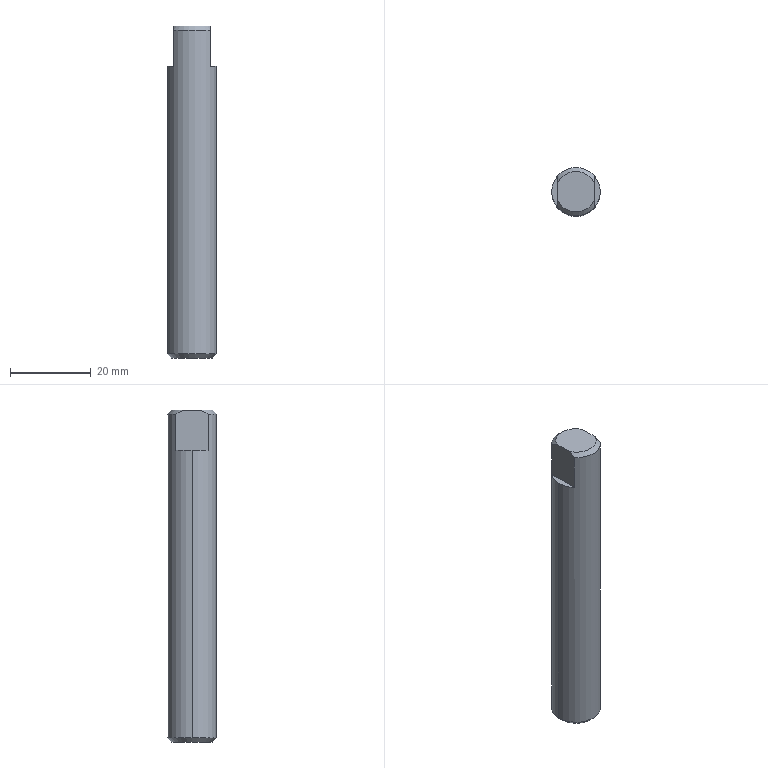Part | STEP file | YCD14007A-08-03.07.07 Sensing Rod | 1 solid | 12 faces | box 12 x 12 x 82 mm | volume 9083 mm3 | plane 6 | cone 4 | cylinder 2 | commonest cylinder face diameters 12 x2
STEP:
#1=CARTESIAN_POINT('',(0.,0.,0.));
#2=DIRECTION('',(0.,0.,1.));
#3=DIRECTION('',(1.,0.,0.));
#4=AXIS2_PLACEMENT_3D('',#1,#2,#3);
#5=CARTESIAN_POINT('',(-5.,0.,0.));
#6=VERTEX_POINT('',#5);
#7=CARTESIAN_POINT('',(5.,0.,0.));
#8=VERTEX_POINT('',#7);
#9=CARTESIAN_POINT('',(0.,0.,0.));
#10=DIRECTION('',(0.,0.,-1.));
#11=DIRECTION('',(1.,0.,0.));
#12=AXIS2_PLACEMENT_3D('',#9,#10,#11);
#13=CIRCLE('',#12,5.);
#14=CARTESIAN_POINT('',(0.,0.,1.));
#15=DIRECTION('',(0.,0.,1.));
#16=DIRECTION('',(1.,0.,0.));
#17=AXIS2_PLACEMENT_3D('',#14,#15,#16);
#18=CONICAL_SURFACE('',#17,6.,0.7854);
#19=CARTESIAN_POINT('',(6.283,-1.));
#20=DIRECTION('',(-1.,0.));
#21=VECTOR('',#20,1.);
#22=LINE('',#19,#21);
#23=(GEOMETRIC_REPRESENTATION_CONTEXT(2)PARAMETRIC_REPRESENTATION_CONTEXT()REPRESENTATION_CONTEXT('',''));
#24=DEFINITIONAL_REPRESENTATION('',(#22),#23);
#25=PCURVE('',#18,#24);
#26=CARTESIAN_POINT('',(0.,0.,0.));
#27=DIRECTION('',(0.,0.,1.));
#28=DIRECTION('',(1.,0.,0.));
#29=AXIS2_PLACEMENT_3D('',#26,#27,#28);
#30=PLANE('',#29);
#31=CARTESIAN_POINT('',(5.,0.));
#32=CARTESIAN_POINT('',(5.,-8.66));
#33=CARTESIAN_POINT('',(-2.5,-4.33));
#34=CARTESIAN_POINT('',(-10.,0.));
#35=CARTESIAN_POINT('',(-2.5,4.33));
#36=CARTESIAN_POINT('',(5.,8.66));
#37=CARTESIAN_POINT('',(5.,0.));
#38=(BOUNDED_CURVE()B_SPLINE_CURVE(2,(#31,#32,#33,#34,#35,#36,#37),.UNSPECIFIED.,.T.,.F.)B_SPLINE_CURVE_WITH_KNOTS((1,2,2,2,2,1),(-2.094,0.,2.094,4.189,6.283,8.378),.UNSPECIFIED.)CURVE()GEOMETRIC_REPRESENTATION_ITEM()RATIONAL_B_SPLINE_CURVE((1.,0.5,1.,0.5,1.,0.5,1.))REPRESENTATION_ITEM(''));
#39=(GEOMETRIC_REPRESENTATION_CONTEXT(2)PARAMETRIC_REPRESENTATION_CONTEXT()REPRESENTATION_CONTEXT('',''));
#40=DEFINITIONAL_REPRESENTATION('',(#38),#39);
#41=PCURVE('',#30,#40);
#42=SURFACE_CURVE('',#13,(#25,#41),.PCURVE_S1.);
#43=EDGE_CURVE('',#6,#8,#42,.T.);
#44=ORIENTED_EDGE('',*,*,#43,.F.);
#45=CARTESIAN_POINT('',(-6.,0.,1.));
#46=VERTEX_POINT('',#45);
#47=CARTESIAN_POINT('',(-6.,0.,1.));
#48=DIRECTION('',(-0.7071,0.,0.7071));
#49=VECTOR('',#48,1.);
#50=LINE('',#47,#49);
#51=CARTESIAN_POINT('',(3.142,0.));
#52=DIRECTION('',(0.,1.));
#53=VECTOR('',#52,1.);
#54=LINE('',#51,#53);
#55=(GEOMETRIC_REPRESENTATION_CONTEXT(2)PARAMETRIC_REPRESENTATION_CONTEXT()REPRESENTATION_CONTEXT('',''));
#56=DEFINITIONAL_REPRESENTATION('',(#54),#55);
#57=PCURVE('',#18,#56);
#58=CARTESIAN_POINT('',(0.,0.,1.));
#59=DIRECTION('',(0.,0.,1.));
#60=DIRECTION('',(1.,0.,0.));
#61=AXIS2_PLACEMENT_3D('',#58,#59,#60);
#62=CONICAL_SURFACE('',#61,6.,0.7854);
#63=CARTESIAN_POINT('',(3.142,0.));
#64=DIRECTION('',(0.,1.));
#65=VECTOR('',#64,1.);
#66=LINE('',#63,#65);
#67=(GEOMETRIC_REPRESENTATION_CONTEXT(2)PARAMETRIC_REPRESENTATION_CONTEXT()REPRESENTATION_CONTEXT('',''));
#68=DEFINITIONAL_REPRESENTATION('',(#66),#67);
#69=PCURVE('',#62,#68);
#70=SURFACE_CURVE('',#50,(#57,#69),.PCURVE_S1.);
#71=EDGE_CURVE('',#6,#46,#70,.T.);
#72=ORIENTED_EDGE('',*,*,#71,.T.);
#73=CARTESIAN_POINT('',(6.,0.,1.));
#74=VERTEX_POINT('',#73);
#75=CARTESIAN_POINT('',(0.,0.,1.));
#76=DIRECTION('',(0.,0.,1.));
#77=DIRECTION('',(1.,0.,0.));
#78=AXIS2_PLACEMENT_3D('',#75,#76,#77);
#79=CIRCLE('',#78,6.);
#80=CARTESIAN_POINT('',(0.,0.));
#81=DIRECTION('',(1.,0.));
#82=VECTOR('',#81,1.);
#83=LINE('',#80,#82);
#84=(GEOMETRIC_REPRESENTATION_CONTEXT(2)PARAMETRIC_REPRESENTATION_CONTEXT()REPRESENTATION_CONTEXT('',''));
#85=DEFINITIONAL_REPRESENTATION('',(#83),#84);
#86=PCURVE('',#18,#85);
#87=CARTESIAN_POINT('',(0.,0.,82.));
#88=DIRECTION('',(0.,0.,-1.));
#89=DIRECTION('',(-1.,0.,0.));
#90=AXIS2_PLACEMENT_3D('',#87,#88,#89);
#91=CYLINDRICAL_SURFACE('',#90,6.);
#92=CARTESIAN_POINT('',(3.142,81.));
#93=DIRECTION('',(-1.,0.));
#94=VECTOR('',#93,1.);
#95=LINE('',#92,#94);
#96=(GEOMETRIC_REPRESENTATION_CONTEXT(2)PARAMETRIC_REPRESENTATION_CONTEXT()REPRESENTATION_CONTEXT('',''));
#97=DEFINITIONAL_REPRESENTATION('',(#95),#96);
#98=PCURVE('',#91,#97);
#99=SURFACE_CURVE('',#79,(#86,#98),.PCURVE_S1.);
#100=EDGE_CURVE('',#74,#46,#99,.T.);
#101=ORIENTED_EDGE('',*,*,#100,.F.);
#102=CARTESIAN_POINT('',(6.,0.,1.));
#103=DIRECTION('',(0.7071,0.,0.7071));
#104=VECTOR('',#103,1.);
#105=LINE('',#102,#104);
#106=CARTESIAN_POINT('',(0.,0.));
#107=DIRECTION('',(0.,1.));
#108=VECTOR('',#107,1.);
#109=LINE('',#106,#108);
#110=(GEOMETRIC_REPRESENTATION_CONTEXT(2)PARAMETRIC_REPRESENTATION_CONTEXT()REPRESENTATION_CONTEXT('',''));
#111=DEFINITIONAL_REPRESENTATION('',(#109),#110);
#112=PCURVE('',#18,#111);
#113=CARTESIAN_POINT('',(6.283,0.));
#114=DIRECTION('',(0.,1.));
#115=VECTOR('',#114,1.);
#116=LINE('',#113,#115);
#117=(GEOMETRIC_REPRESENTATION_CONTEXT(2)PARAMETRIC_REPRESENTATION_CONTEXT()REPRESENTATION_CONTEXT('',''));
#118=DEFINITIONAL_REPRESENTATION('',(#116),#117);
#119=PCURVE('',#62,#118);
#120=SURFACE_CURVE('',#105,(#112,#119),.PCURVE_S1.);
#121=EDGE_CURVE('',#8,#74,#120,.T.);
#122=ORIENTED_EDGE('',*,*,#121,.F.);
#123=EDGE_LOOP('',(#44,#72,#101,#122));
#124=FACE_BOUND('',#123,.T.);
#125=ADVANCED_FACE('',(#124),#18,.T.);
#126=CARTESIAN_POINT('',(4.5,3.969,72.));
#127=VERTEX_POINT('',#126);
#128=CARTESIAN_POINT('',(6.,0.,72.));
#129=VERTEX_POINT('',#128);
#130=CARTESIAN_POINT('',(0.,0.,72.));
#131=DIRECTION('',(0.,0.,-1.));
#132=DIRECTION('',(-1.,0.,0.));
#133=AXIS2_PLACEMENT_3D('',#130,#131,#132);
#134=CIRCLE('',#133,6.);
#135=CARTESIAN_POINT('',(0.,10.));
#136=DIRECTION('',(1.,0.));
#137=VECTOR('',#136,1.);
#138=LINE('',#135,#137);
#139=(GEOMETRIC_REPRESENTATION_CONTEXT(2)PARAMETRIC_REPRESENTATION_CONTEXT()REPRESENTATION_CONTEXT('',''));
#140=DEFINITIONAL_REPRESENTATION('',(#138),#139);
#141=PCURVE('',#91,#140);
#142=CARTESIAN_POINT('',(6.,-32.,72.));
#143=DIRECTION('',(0.,0.,-1.));
#144=DIRECTION('',(-1.,0.,0.));
#145=AXIS2_PLACEMENT_3D('',#142,#143,#144);
#146=PLANE('',#145);
#147=CARTESIAN_POINT('',(6.,32.));
#148=DIRECTION('',(1.,0.));
#149=AXIS2_PLACEMENT_2D('',#147,#148);
#150=CIRCLE('',#149,6.);
#151=(GEOMETRIC_REPRESENTATION_CONTEXT(2)PARAMETRIC_REPRESENTATION_CONTEXT()REPRESENTATION_CONTEXT('',''));
#152=DEFINITIONAL_REPRESENTATION('',(#150),#151);
#153=PCURVE('',#146,#152);
#154=SURFACE_CURVE('',#134,(#141,#153),.PCURVE_S1.);
#155=EDGE_CURVE('',#127,#129,#154,.T.);
#156=ORIENTED_EDGE('',*,*,#155,.T.);
#157=CARTESIAN_POINT('',(6.,0.,82.));
#158=DIRECTION('',(0.,0.,-1.));
#159=VECTOR('',#158,1.);
#160=LINE('',#157,#159);
#161=CARTESIAN_POINT('',(3.142,0.));
#162=DIRECTION('',(0.,1.));
#163=VECTOR('',#162,1.);
#164=LINE('',#161,#163);
#165=(GEOMETRIC_REPRESENTATION_CONTEXT(2)PARAMETRIC_REPRESENTATION_CONTEXT()REPRESENTATION_CONTEXT('',''));
#166=DEFINITIONAL_REPRESENTATION('',(#164),#165);
#167=PCURVE('',#91,#166);
#168=CARTESIAN_POINT('',(0.,0.,82.));
#169=DIRECTION('',(0.,0.,-1.));
#170=DIRECTION('',(-1.,0.,0.));
#171=AXIS2_PLACEMENT_3D('',#168,#169,#170);
#172=CYLINDRICAL_SURFACE('',#171,6.);
#173=CARTESIAN_POINT('',(3.142,0.));
#174=DIRECTION('',(0.,1.));
#175=VECTOR('',#174,1.);
#176=LINE('',#173,#175);
#177=(GEOMETRIC_REPRESENTATION_CONTEXT(2)PARAMETRIC_REPRESENTATION_CONTEXT()REPRESENTATION_CONTEXT('',''));
#178=DEFINITIONAL_REPRESENTATION('',(#176),#177);
#179=PCURVE('',#172,#178);
#180=SURFACE_CURVE('',#160,(#167,#179),.PCURVE_S1.);
#181=EDGE_CURVE('',#129,#74,#180,.T.);
#182=ORIENTED_EDGE('',*,*,#181,.T.);
#183=ORIENTED_EDGE('',*,*,#100,.T.);
#184=CARTESIAN_POINT('',(-6.,0.,72.));
#185=VERTEX_POINT('',#184);
#186=CARTESIAN_POINT('',(-6.,0.,82.));
#187=DIRECTION('',(0.,0.,-1.));
#188=VECTOR('',#187,1.);
#189=LINE('',#186,#188);
#190=CARTESIAN_POINT('',(0.,0.));
#191=DIRECTION('',(0.,1.));
#192=VECTOR('',#191,1.);
#193=LINE('',#190,#192);
#194=(GEOMETRIC_REPRESENTATION_CONTEXT(2)PARAMETRIC_REPRESENTATION_CONTEXT()REPRESENTATION_CONTEXT('',''));
#195=DEFINITIONAL_REPRESENTATION('',(#193),#194);
#196=PCURVE('',#91,#195);
#197=CARTESIAN_POINT('',(6.283,0.));
#198=DIRECTION('',(0.,1.));
#199=VECTOR('',#198,1.);
#200=LINE('',#197,#199);
#201=(GEOMETRIC_REPRESENTATION_CONTEXT(2)PARAMETRIC_REPRESENTATION_CONTEXT()REPRESENTATION_CONTEXT('',''));
#202=DEFINITIONAL_REPRESENTATION('',(#200),#201);
#203=PCURVE('',#172,#202);
#204=SURFACE_CURVE('',#189,(#196,#203),.PCURVE_S1.);
#205=EDGE_CURVE('',#185,#46,#204,.T.);
#206=ORIENTED_EDGE('',*,*,#205,.F.);
#207=CARTESIAN_POINT('',(-4.5,3.969,72.));
#208=VERTEX_POINT('',#207);
#209=CARTESIAN_POINT('',(0.,0.,72.));
#210=DIRECTION('',(0.,0.,-1.));
#211=DIRECTION('',(-1.,0.,0.));
#212=AXIS2_PLACEMENT_3D('',#209,#210,#211);
#213=CIRCLE('',#212,6.);
#214=CARTESIAN_POINT('',(0.,10.));
#215=DIRECTION('',(1.,0.));
#216=VECTOR('',#215,1.);
#217=LINE('',#214,#216);
#218=(GEOMETRIC_REPRESENTATION_CONTEXT(2)PARAMETRIC_REPRESENTATION_CONTEXT()REPRESENTATION_CONTEXT('',''));
#219=DEFINITIONAL_REPRESENTATION('',(#217),#218);
#220=PCURVE('',#91,#219);
#221=CARTESIAN_POINT('',(-6.,-32.,72.));
#222=DIRECTION('',(0.,0.,-1.));
#223=DIRECTION('',(-1.,0.,0.));
#224=AXIS2_PLACEMENT_3D('',#221,#222,#223);
#225=PLANE('',#224);
#226=CARTESIAN_POINT('',(-6.,32.));
#227=DIRECTION('',(1.,0.));
#228=AXIS2_PLACEMENT_2D('',#226,#227);
#229=CIRCLE('',#228,6.);
#230=(GEOMETRIC_REPRESENTATION_CONTEXT(2)PARAMETRIC_REPRESENTATION_CONTEXT()REPRESENTATION_CONTEXT('',''));
#231=DEFINITIONAL_REPRESENTATION('',(#229),#230);
#232=PCURVE('',#225,#231);
#233=SURFACE_CURVE('',#213,(#220,#232),.PCURVE_S1.);
#234=EDGE_CURVE('',#185,#208,#233,.T.);
#235=ORIENTED_EDGE('',*,*,#234,.T.);
#236=CARTESIAN_POINT('',(-4.5,3.969,81.));
#237=VERTEX_POINT('',#236);
#238=CARTESIAN_POINT('',(-4.5,3.969,82.));
#239=DIRECTION('',(0.,0.,1.));
#240=VECTOR('',#239,1.);
#241=LINE('',#238,#240);
#242=CARTESIAN_POINT('',(0.7227,0.));
#243=DIRECTION('',(0.,-1.));
#244=VECTOR('',#243,1.);
#245=LINE('',#242,#244);
#246=(GEOMETRIC_REPRESENTATION_CONTEXT(2)PARAMETRIC_REPRESENTATION_CONTEXT()REPRESENTATION_CONTEXT('',''));
#247=DEFINITIONAL_REPRESENTATION('',(#245),#246);
#248=PCURVE('',#91,#247);
#249=CARTESIAN_POINT('',(-4.5,-32.,82.));
#250=DIRECTION('',(1.,0.,0.));
#251=DIRECTION('',(0.,0.,-1.));
#252=AXIS2_PLACEMENT_3D('',#249,#250,#251);
#253=PLANE('',#252);
#254=CARTESIAN_POINT('',(0.,35.969));
#255=DIRECTION('',(-1.,0.));
#256=VECTOR('',#255,1.);
#257=LINE('',#254,#256);
#258=(GEOMETRIC_REPRESENTATION_CONTEXT(2)PARAMETRIC_REPRESENTATION_CONTEXT()REPRESENTATION_CONTEXT('',''));
#259=DEFINITIONAL_REPRESENTATION('',(#257),#258);
#260=PCURVE('',#253,#259);
#261=SURFACE_CURVE('',#241,(#248,#260),.PCURVE_S1.);
#262=EDGE_CURVE('',#208,#237,#261,.T.);
#263=ORIENTED_EDGE('',*,*,#262,.T.);
#264=CARTESIAN_POINT('',(4.5,3.969,81.));
#265=VERTEX_POINT('',#264);
#266=CARTESIAN_POINT('',(0.,0.,81.));
#267=DIRECTION('',(0.,0.,-1.));
#268=DIRECTION('',(1.,0.,0.));
#269=AXIS2_PLACEMENT_3D('',#266,#267,#268);
#270=CIRCLE('',#269,6.);
#271=CARTESIAN_POINT('',(-3.142,1.));
#272=DIRECTION('',(1.,0.));
#273=VECTOR('',#272,1.);
#274=LINE('',#271,#273);
#275=(GEOMETRIC_REPRESENTATION_CONTEXT(2)PARAMETRIC_REPRESENTATION_CONTEXT()REPRESENTATION_CONTEXT('',''));
#276=DEFINITIONAL_REPRESENTATION('',(#274),#275);
#277=PCURVE('',#91,#276);
#278=CARTESIAN_POINT('',(0.,0.,82.));
#279=DIRECTION('',(0.,0.,-1.));
#280=DIRECTION('',(-1.,0.,0.));
#281=AXIS2_PLACEMENT_3D('',#278,#279,#280);
#282=CONICAL_SURFACE('',#281,5.,0.7854);
#283=CARTESIAN_POINT('',(-3.142,1.));
#284=DIRECTION('',(1.,0.));
#285=VECTOR('',#284,1.);
#286=LINE('',#283,#285);
#287=(GEOMETRIC_REPRESENTATION_CONTEXT(2)PARAMETRIC_REPRESENTATION_CONTEXT()REPRESENTATION_CONTEXT('',''));
#288=DEFINITIONAL_REPRESENTATION('',(#286),#287);
#289=PCURVE('',#282,#288);
#290=SURFACE_CURVE('',#270,(#277,#289),.PCURVE_S1.);
#291=EDGE_CURVE('',#237,#265,#290,.T.);
#292=ORIENTED_EDGE('',*,*,#291,.T.);
#293=CARTESIAN_POINT('',(4.5,3.969,82.));
#294=DIRECTION('',(0.,0.,-1.));
#295=VECTOR('',#294,1.);
#296=LINE('',#293,#295);
#297=CARTESIAN_POINT('',(2.419,0.));
#298=DIRECTION('',(0.,1.));
#299=VECTOR('',#298,1.);
#300=LINE('',#297,#299);
#301=(GEOMETRIC_REPRESENTATION_CONTEXT(2)PARAMETRIC_REPRESENTATION_CONTEXT()REPRESENTATION_CONTEXT('',''));
#302=DEFINITIONAL_REPRESENTATION('',(#300),#301);
#303=PCURVE('',#91,#302);
#304=CARTESIAN_POINT('',(4.5,-32.,82.));
#305=DIRECTION('',(-1.,0.,0.));
#306=DIRECTION('',(0.,0.,1.));
#307=AXIS2_PLACEMENT_3D('',#304,#305,#306);
#308=PLANE('',#307);
#309=CARTESIAN_POINT('',(0.,35.969));
#310=DIRECTION('',(-1.,0.));
#311=VECTOR('',#310,1.);
#312=LINE('',#309,#311);
#313=(GEOMETRIC_REPRESENTATION_CONTEXT(2)PARAMETRIC_REPRESENTATION_CONTEXT()REPRESENTATION_CONTEXT('',''));
#314=DEFINITIONAL_REPRESENTATION('',(#312),#313);
#315=PCURVE('',#308,#314);
#316=SURFACE_CURVE('',#296,(#303,#315),.PCURVE_S1.);
#317=EDGE_CURVE('',#265,#127,#316,.T.);
#318=ORIENTED_EDGE('',*,*,#317,.T.);
#319=EDGE_LOOP('',(#156,#182,#183,#206,#235,#263,#292,#318));
#320=FACE_BOUND('',#319,.T.);
#321=ADVANCED_FACE('',(#320),#91,.T.);
#322=CARTESIAN_POINT('',(-4.5,-3.969,81.));
#323=VERTEX_POINT('',#322);
#324=CARTESIAN_POINT('',(-4.5,-2.179,82.));
#325=VERTEX_POINT('',#324);
#326=CARTESIAN_POINT('',(-4.5,-3.969,81.));
#327=CARTESIAN_POINT('',(-4.5,-3.685,81.187));
#328=CARTESIAN_POINT('',(-4.5,-3.396,81.367));
#329=CARTESIAN_POINT('',(-4.5,-2.802,81.704));
#330=CARTESIAN_POINT('',(-4.5,-2.497,81.862));
#331=CARTESIAN_POINT('',(-4.5,-2.179,82.));
#332=B_SPLINE_CURVE_WITH_KNOTS('',3,(#326,#327,#328,#329,#330,#331),.UNSPECIFIED.,.F.,.F.,(4,2,4),(0.01115,0.01218,0.0132),.UNSPECIFIED.);
#333=CARTESIAN_POINT('',(0.,0.,82.));
#334=DIRECTION('',(0.,0.,-1.));
#335=DIRECTION('',(-1.,0.,0.));
#336=AXIS2_PLACEMENT_3D('',#333,#334,#335);
#337=CONICAL_SURFACE('',#336,5.,0.7854);
#338=CARTESIAN_POINT('',(5.56,1.));
#339=CARTESIAN_POINT('',(5.564,0.983));
#340=CARTESIAN_POINT('',(5.57,0.949));
#341=CARTESIAN_POINT('',(5.58,0.8984));
#342=CARTESIAN_POINT('',(5.59,0.8483));
#343=CARTESIAN_POINT('',(5.601,0.7986));
#344=CARTESIAN_POINT('',(5.611,0.7493));
#345=CARTESIAN_POINT('',(5.622,0.7005));
#346=CARTESIAN_POINT('',(5.633,0.6522));
#347=CARTESIAN_POINT('',(5.645,0.6044));
#348=CARTESIAN_POINT('',(5.656,0.557));
#349=CARTESIAN_POINT('',(5.668,0.5103));
#350=CARTESIAN_POINT('',(5.68,0.464));
#351=CARTESIAN_POINT('',(5.692,0.4184));
#352=CARTESIAN_POINT('',(5.705,0.3733));
#353=CARTESIAN_POINT('',(5.718,0.3288));
#354=CARTESIAN_POINT('',(5.731,0.285));
#355=CARTESIAN_POINT('',(5.745,0.2419));
#356=CARTESIAN_POINT('',(5.758,0.1996));
#357=CARTESIAN_POINT('',(5.772,0.1579));
#358=CARTESIAN_POINT('',(5.787,0.1171));
#359=CARTESIAN_POINT('',(5.802,0.07713));
#360=CARTESIAN_POINT('',(5.817,0.03803));
#361=CARTESIAN_POINT('',(5.827,0.01257));
#362=CARTESIAN_POINT('',(5.832,0.));
#363=B_SPLINE_CURVE_WITH_KNOTS('',3,(#338,#339,#340,#341,#342,#343,#344,#345,#346,#347,#348,#349,#350,#351,#352,#353,#354,#355,#356,#357,#358,#359,#360,#361,#362),.UNSPECIFIED.,.F.,.F.,(4,1,1,1,1,1,1,1,1,1,1,1,1,1,1,1,1,1,1,1,1,1,4),(0.01115,0.01125,0.01134,0.01143,0.01152,0.01162,0.01171,0.0118,0.0119,0.01199,0.01208,0.01218,0.01227,0.01236,0.01245,0.01255,0.01264,0.01273,0.01283,0.01292,0.01301,0.01311,0.0132),.QUASI_UNIFORM_KNOTS.);
#364=(GEOMETRIC_REPRESENTATION_CONTEXT(2)PARAMETRIC_REPRESENTATION_CONTEXT()REPRESENTATION_CONTEXT('',''));
#365=DEFINITIONAL_REPRESENTATION('',(#363),#364);
#366=PCURVE('',#337,#365);
#367=CARTESIAN_POINT('',(1.,28.031));
#368=CARTESIAN_POINT('',(0.8125,28.315));
#369=CARTESIAN_POINT('',(0.6326,28.604));
#370=CARTESIAN_POINT('',(0.2957,29.198));
#371=CARTESIAN_POINT('',(0.1383,29.503));
#372=CARTESIAN_POINT('',(0.,29.821));
#373=B_SPLINE_CURVE_WITH_KNOTS('',3,(#367,#368,#369,#370,#371,#372),.UNSPECIFIED.,.F.,.F.,(4,2,4),(0.01115,0.01218,0.0132),.UNSPECIFIED.);
#374=(GEOMETRIC_REPRESENTATION_CONTEXT(2)PARAMETRIC_REPRESENTATION_CONTEXT()REPRESENTATION_CONTEXT('',''));
#375=DEFINITIONAL_REPRESENTATION('',(#373),#374);
#376=PCURVE('',#253,#375);
#377=SURFACE_CURVE('',#332,(#366,#376),.PCURVE_S1.);
#378=EDGE_CURVE('',#323,#325,#377,.T.);
#379=ORIENTED_EDGE('',*,*,#378,.F.);
#380=CARTESIAN_POINT('',(4.5,-3.969,81.));
#381=VERTEX_POINT('',#380);
#382=CARTESIAN_POINT('',(0.,0.,81.));
#383=DIRECTION('',(0.,0.,-1.));
#384=DIRECTION('',(1.,0.,0.));
#385=AXIS2_PLACEMENT_3D('',#382,#383,#384);
#386=CIRCLE('',#385,6.);
#387=CARTESIAN_POINT('',(3.142,1.));
#388=DIRECTION('',(1.,0.));
#389=VECTOR('',#388,1.);
#390=LINE('',#387,#389);
#391=(GEOMETRIC_REPRESENTATION_CONTEXT(2)PARAMETRIC_REPRESENTATION_CONTEXT()REPRESENTATION_CONTEXT('',''));
#392=DEFINITIONAL_REPRESENTATION('',(#390),#391);
#393=PCURVE('',#337,#392);
#394=CARTESIAN_POINT('',(3.142,1.));
#395=DIRECTION('',(1.,0.));
#396=VECTOR('',#395,1.);
#397=LINE('',#394,#396);
#398=(GEOMETRIC_REPRESENTATION_CONTEXT(2)PARAMETRIC_REPRESENTATION_CONTEXT()REPRESENTATION_CONTEXT('',''));
#399=DEFINITIONAL_REPRESENTATION('',(#397),#398);
#400=PCURVE('',#172,#399);
#401=SURFACE_CURVE('',#386,(#393,#400),.PCURVE_S1.);
#402=EDGE_CURVE('',#381,#323,#401,.T.);
#403=ORIENTED_EDGE('',*,*,#402,.F.);
#404=CARTESIAN_POINT('',(4.5,-2.179,82.));
#405=VERTEX_POINT('',#404);
#406=CARTESIAN_POINT('',(4.5,-2.179,82.));
#407=CARTESIAN_POINT('',(4.5,-2.492,81.864));
#408=CARTESIAN_POINT('',(4.5,-2.796,81.708));
#409=CARTESIAN_POINT('',(4.5,-3.391,81.371));
#410=CARTESIAN_POINT('',(4.5,-3.683,81.189));
#411=CARTESIAN_POINT('',(4.5,-3.969,81.));
#412=B_SPLINE_CURVE_WITH_KNOTS('',3,(#406,#407,#408,#409,#410,#411),.UNSPECIFIED.,.F.,.F.,(4,2,4),(0.01766,0.01868,0.0197),.UNSPECIFIED.);
#413=CARTESIAN_POINT('',(3.593,0.));
#414=CARTESIAN_POINT('',(3.598,0.01239));
#415=CARTESIAN_POINT('',(3.608,0.03749));
#416=CARTESIAN_POINT('',(3.623,0.07609));
#417=CARTESIAN_POINT('',(3.637,0.1156));
#418=CARTESIAN_POINT('',(3.652,0.156));
#419=CARTESIAN_POINT('',(3.666,0.1972));
#420=CARTESIAN_POINT('',(3.679,0.2392));
#421=CARTESIAN_POINT('',(3.693,0.2821));
#422=CARTESIAN_POINT('',(3.706,0.3256));
#423=CARTESIAN_POINT('',(3.719,0.3699));
#424=CARTESIAN_POINT('',(3.731,0.4149));
#425=CARTESIAN_POINT('',(3.744,0.4606));
#426=CARTESIAN_POINT('',(3.756,0.5069));
#427=CARTESIAN_POINT('',(3.768,0.5539));
#428=CARTESIAN_POINT('',(3.78,0.6014));
#429=CARTESIAN_POINT('',(3.791,0.6496));
#430=CARTESIAN_POINT('',(3.802,0.6982));
#431=CARTESIAN_POINT('',(3.813,0.7474));
#432=CARTESIAN_POINT('',(3.824,0.7971));
#433=CARTESIAN_POINT('',(3.834,0.8472));
#434=CARTESIAN_POINT('',(3.844,0.8977));
#435=CARTESIAN_POINT('',(3.855,0.9487));
#436=CARTESIAN_POINT('',(3.861,0.9828));
#437=CARTESIAN_POINT('',(3.864,1.));
#438=B_SPLINE_CURVE_WITH_KNOTS('',3,(#413,#414,#415,#416,#417,#418,#419,#420,#421,#422,#423,#424,#425,#426,#427,#428,#429,#430,#431,#432,#433,#434,#435,#436,#437),.UNSPECIFIED.,.F.,.F.,(4,1,1,1,1,1,1,1,1,1,1,1,1,1,1,1,1,1,1,1,1,1,4),(0.01766,0.01776,0.01785,0.01794,0.01804,0.01813,0.01822,0.01831,0.01841,0.0185,0.01859,0.01868,0.01878,0.01887,0.01896,0.01905,0.01915,0.01924,0.01933,0.01942,0.01952,0.01961,0.0197),.QUASI_UNIFORM_KNOTS.);
#439=(GEOMETRIC_REPRESENTATION_CONTEXT(2)PARAMETRIC_REPRESENTATION_CONTEXT()REPRESENTATION_CONTEXT('',''));
#440=DEFINITIONAL_REPRESENTATION('',(#438),#439);
#441=PCURVE('',#337,#440);
#442=CARTESIAN_POINT('',(0.,29.821));
#443=CARTESIAN_POINT('',(-0.1363,29.508));
#444=CARTESIAN_POINT('',(-0.2921,29.204));
#445=CARTESIAN_POINT('',(-0.6294,28.609));
#446=CARTESIAN_POINT('',(-0.8113,28.317));
#447=CARTESIAN_POINT('',(-1.,28.031));
#448=B_SPLINE_CURVE_WITH_KNOTS('',3,(#442,#443,#444,#445,#446,#447),.UNSPECIFIED.,.F.,.F.,(4,2,4),(0.01766,0.01868,0.0197),.UNSPECIFIED.);
#449=(GEOMETRIC_REPRESENTATION_CONTEXT(2)PARAMETRIC_REPRESENTATION_CONTEXT()REPRESENTATION_CONTEXT('',''));
#450=DEFINITIONAL_REPRESENTATION('',(#448),#449);
#451=PCURVE('',#308,#450);
#452=SURFACE_CURVE('',#412,(#441,#451),.PCURVE_S1.);
#453=EDGE_CURVE('',#405,#381,#452,.T.);
#454=ORIENTED_EDGE('',*,*,#453,.F.);
#455=CARTESIAN_POINT('',(0.,0.,82.));
#456=DIRECTION('',(0.,0.,1.));
#457=DIRECTION('',(1.,0.,0.));
#458=AXIS2_PLACEMENT_3D('',#455,#456,#457);
#459=CIRCLE('',#458,5.);
#460=CARTESIAN_POINT('',(9.425,0.));
#461=DIRECTION('',(-1.,0.));
#462=VECTOR('',#461,1.);
#463=LINE('',#460,#462);
#464=(GEOMETRIC_REPRESENTATION_CONTEXT(2)PARAMETRIC_REPRESENTATION_CONTEXT()REPRESENTATION_CONTEXT('',''));
#465=DEFINITIONAL_REPRESENTATION('',(#463),#464);
#466=PCURVE('',#337,#465);
#467=CARTESIAN_POINT('',(0.,0.,82.));
#468=DIRECTION('',(0.,0.,1.));
#469=DIRECTION('',(1.,0.,0.));
#470=AXIS2_PLACEMENT_3D('',#467,#468,#469);
#471=PLANE('',#470);
#472=CARTESIAN_POINT('',(0.,0.));
#473=DIRECTION('',(1.,0.));
#474=AXIS2_PLACEMENT_2D('',#472,#473);
#475=CIRCLE('',#474,5.);
#476=(GEOMETRIC_REPRESENTATION_CONTEXT(2)PARAMETRIC_REPRESENTATION_CONTEXT()REPRESENTATION_CONTEXT('',''));
#477=DEFINITIONAL_REPRESENTATION('',(#475),#476);
#478=PCURVE('',#471,#477);
#479=SURFACE_CURVE('',#459,(#466,#478),.PCURVE_S1.);
#480=EDGE_CURVE('',#325,#405,#479,.T.);
#481=ORIENTED_EDGE('',*,*,#480,.F.);
#482=EDGE_LOOP('',(#379,#403,#454,#481));
#483=FACE_BOUND('',#482,.T.);
#484=ADVANCED_FACE('',(#483),#337,.T.);
#485=ORIENTED_EDGE('',*,*,#181,.F.);
#486=CARTESIAN_POINT('',(4.5,-3.969,72.));
#487=VERTEX_POINT('',#486);
#488=CARTESIAN_POINT('',(0.,0.,72.));
#489=DIRECTION('',(0.,0.,-1.));
#490=DIRECTION('',(-1.,0.,0.));
#491=AXIS2_PLACEMENT_3D('',#488,#489,#490);
#492=CIRCLE('',#491,6.);
#493=CARTESIAN_POINT('',(0.,10.));
#494=DIRECTION('',(1.,0.));
#495=VECTOR('',#494,1.);
#496=LINE('',#493,#495);
#497=(GEOMETRIC_REPRESENTATION_CONTEXT(2)PARAMETRIC_REPRESENTATION_CONTEXT()REPRESENTATION_CONTEXT('',''));
#498=DEFINITIONAL_REPRESENTATION('',(#496),#497);
#499=PCURVE('',#172,#498);
#500=CARTESIAN_POINT('',(6.,32.));
#501=DIRECTION('',(1.,0.));
#502=AXIS2_PLACEMENT_2D('',#500,#501);
#503=CIRCLE('',#502,6.);
#504=(GEOMETRIC_REPRESENTATION_CONTEXT(2)PARAMETRIC_REPRESENTATION_CONTEXT()REPRESENTATION_CONTEXT('',''));
#505=DEFINITIONAL_REPRESENTATION('',(#503),#504);
#506=PCURVE('',#146,#505);
#507=SURFACE_CURVE('',#492,(#499,#506),.PCURVE_S1.);
#508=EDGE_CURVE('',#129,#487,#507,.T.);
#509=ORIENTED_EDGE('',*,*,#508,.T.);
#510=CARTESIAN_POINT('',(4.5,-3.969,82.));
#511=DIRECTION('',(0.,0.,1.));
#512=VECTOR('',#511,1.);
#513=LINE('',#510,#512);
#514=CARTESIAN_POINT('',(3.864,0.));
#515=DIRECTION('',(0.,-1.));
#516=VECTOR('',#515,1.);
#517=LINE('',#514,#516);
#518=(GEOMETRIC_REPRESENTATION_CONTEXT(2)PARAMETRIC_REPRESENTATION_CONTEXT()REPRESENTATION_CONTEXT('',''));
#519=DEFINITIONAL_REPRESENTATION('',(#517),#518);
#520=PCURVE('',#172,#519);
#521=CARTESIAN_POINT('',(0.,28.031));
#522=DIRECTION('',(1.,0.));
#523=VECTOR('',#522,1.);
#524=LINE('',#521,#523);
#525=(GEOMETRIC_REPRESENTATION_CONTEXT(2)PARAMETRIC_REPRESENTATION_CONTEXT()REPRESENTATION_CONTEXT('',''));
#526=DEFINITIONAL_REPRESENTATION('',(#524),#525);
#527=PCURVE('',#308,#526);
#528=SURFACE_CURVE('',#513,(#520,#527),.PCURVE_S1.);
#529=EDGE_CURVE('',#487,#381,#528,.T.);
#530=ORIENTED_EDGE('',*,*,#529,.T.);
#531=ORIENTED_EDGE('',*,*,#402,.T.);
#532=CARTESIAN_POINT('',(-4.5,-3.969,72.));
#533=VERTEX_POINT('',#532);
#534=CARTESIAN_POINT('',(-4.5,-3.969,82.));
#535=DIRECTION('',(0.,0.,-1.));
#536=VECTOR('',#535,1.);
#537=LINE('',#534,#536);
#538=CARTESIAN_POINT('',(5.56,0.));
#539=DIRECTION('',(0.,1.));
#540=VECTOR('',#539,1.);
#541=LINE('',#538,#540);
#542=(GEOMETRIC_REPRESENTATION_CONTEXT(2)PARAMETRIC_REPRESENTATION_CONTEXT()REPRESENTATION_CONTEXT('',''));
#543=DEFINITIONAL_REPRESENTATION('',(#541),#542);
#544=PCURVE('',#172,#543);
#545=CARTESIAN_POINT('',(0.,28.031));
#546=DIRECTION('',(1.,0.));
#547=VECTOR('',#546,1.);
#548=LINE('',#545,#547);
#549=(GEOMETRIC_REPRESENTATION_CONTEXT(2)PARAMETRIC_REPRESENTATION_CONTEXT()REPRESENTATION_CONTEXT('',''));
#550=DEFINITIONAL_REPRESENTATION('',(#548),#549);
#551=PCURVE('',#253,#550);
#552=SURFACE_CURVE('',#537,(#544,#551),.PCURVE_S1.);
#553=EDGE_CURVE('',#323,#533,#552,.T.);
#554=ORIENTED_EDGE('',*,*,#553,.T.);
#555=CARTESIAN_POINT('',(0.,0.,72.));
#556=DIRECTION('',(0.,0.,-1.));
#557=DIRECTION('',(-1.,0.,0.));
#558=AXIS2_PLACEMENT_3D('',#555,#556,#557);
#559=CIRCLE('',#558,6.);
#560=CARTESIAN_POINT('',(0.,10.));
#561=DIRECTION('',(1.,0.));
#562=VECTOR('',#561,1.);
#563=LINE('',#560,#562);
#564=(GEOMETRIC_REPRESENTATION_CONTEXT(2)PARAMETRIC_REPRESENTATION_CONTEXT()REPRESENTATION_CONTEXT('',''));
#565=DEFINITIONAL_REPRESENTATION('',(#563),#564);
#566=PCURVE('',#172,#565);
#567=CARTESIAN_POINT('',(-6.,32.));
#568=DIRECTION('',(1.,0.));
#569=AXIS2_PLACEMENT_2D('',#567,#568);
#570=CIRCLE('',#569,6.);
#571=(GEOMETRIC_REPRESENTATION_CONTEXT(2)PARAMETRIC_REPRESENTATION_CONTEXT()REPRESENTATION_CONTEXT('',''));
#572=DEFINITIONAL_REPRESENTATION('',(#570),#571);
#573=PCURVE('',#225,#572);
#574=SURFACE_CURVE('',#559,(#566,#573),.PCURVE_S1.);
#575=EDGE_CURVE('',#533,#185,#574,.T.);
#576=ORIENTED_EDGE('',*,*,#575,.T.);
#577=ORIENTED_EDGE('',*,*,#205,.T.);
#578=CARTESIAN_POINT('',(0.,0.,1.));
#579=DIRECTION('',(0.,0.,1.));
#580=DIRECTION('',(1.,0.,0.));
#581=AXIS2_PLACEMENT_3D('',#578,#579,#580);
#582=CIRCLE('',#581,6.);
#583=CARTESIAN_POINT('',(9.425,81.));
#584=DIRECTION('',(-1.,0.));
#585=VECTOR('',#584,1.);
#586=LINE('',#583,#585);
#587=(GEOMETRIC_REPRESENTATION_CONTEXT(2)PARAMETRIC_REPRESENTATION_CONTEXT()REPRESENTATION_CONTEXT('',''));
#588=DEFINITIONAL_REPRESENTATION('',(#586),#587);
#589=PCURVE('',#172,#588);
#590=CARTESIAN_POINT('',(0.,0.));
#591=DIRECTION('',(1.,0.));
#592=VECTOR('',#591,1.);
#593=LINE('',#590,#592);
#594=(GEOMETRIC_REPRESENTATION_CONTEXT(2)PARAMETRIC_REPRESENTATION_CONTEXT()REPRESENTATION_CONTEXT('',''));
#595=DEFINITIONAL_REPRESENTATION('',(#593),#594);
#596=PCURVE('',#62,#595);
#597=SURFACE_CURVE('',#582,(#589,#596),.PCURVE_S1.);
#598=EDGE_CURVE('',#46,#74,#597,.T.);
#599=ORIENTED_EDGE('',*,*,#598,.T.);
#600=EDGE_LOOP('',(#485,#509,#530,#531,#554,#576,#577,#599));
#601=FACE_BOUND('',#600,.T.);
#602=ADVANCED_FACE('',(#601),#172,.T.);
#603=CARTESIAN_POINT('',(-4.5,2.179,82.));
#604=VERTEX_POINT('',#603);
#605=CARTESIAN_POINT('',(-4.5,-32.,82.));
#606=DIRECTION('',(0.,1.,0.));
#607=VECTOR('',#606,1.);
#608=LINE('',#605,#607);
#609=CARTESIAN_POINT('',(-4.5,-32.));
#610=DIRECTION('',(0.,1.));
#611=VECTOR('',#610,1.);
#612=LINE('',#609,#611);
#613=(GEOMETRIC_REPRESENTATION_CONTEXT(2)PARAMETRIC_REPRESENTATION_CONTEXT()REPRESENTATION_CONTEXT('',''));
#614=DEFINITIONAL_REPRESENTATION('',(#612),#613);
#615=PCURVE('',#471,#614);
#616=CARTESIAN_POINT('',(0.,0.));
#617=DIRECTION('',(0.,1.));
#618=VECTOR('',#617,1.);
#619=LINE('',#616,#618);
#620=(GEOMETRIC_REPRESENTATION_CONTEXT(2)PARAMETRIC_REPRESENTATION_CONTEXT()REPRESENTATION_CONTEXT('',''));
#621=DEFINITIONAL_REPRESENTATION('',(#619),#620);
#622=PCURVE('',#253,#621);
#623=SURFACE_CURVE('',#608,(#615,#622),.PCURVE_S1.);
#624=EDGE_CURVE('',#325,#604,#623,.T.);
#625=ORIENTED_EDGE('',*,*,#624,.F.);
#626=ORIENTED_EDGE('',*,*,#480,.T.);
#627=CARTESIAN_POINT('',(4.5,2.179,82.));
#628=VERTEX_POINT('',#627);
#629=CARTESIAN_POINT('',(4.5,-32.,82.));
#630=DIRECTION('',(0.,1.,0.));
#631=VECTOR('',#630,1.);
#632=LINE('',#629,#631);
#633=CARTESIAN_POINT('',(4.5,-32.));
#634=DIRECTION('',(0.,1.));
#635=VECTOR('',#634,1.);
#636=LINE('',#633,#635);
#637=(GEOMETRIC_REPRESENTATION_CONTEXT(2)PARAMETRIC_REPRESENTATION_CONTEXT()REPRESENTATION_CONTEXT('',''));
#638=DEFINITIONAL_REPRESENTATION('',(#636),#637);
#639=PCURVE('',#471,#638);
#640=CARTESIAN_POINT('',(0.,0.));
#641=DIRECTION('',(0.,1.));
#642=VECTOR('',#641,1.);
#643=LINE('',#640,#642);
#644=(GEOMETRIC_REPRESENTATION_CONTEXT(2)PARAMETRIC_REPRESENTATION_CONTEXT()REPRESENTATION_CONTEXT('',''));
#645=DEFINITIONAL_REPRESENTATION('',(#643),#644);
#646=PCURVE('',#308,#645);
#647=SURFACE_CURVE('',#632,(#639,#646),.PCURVE_S1.);
#648=EDGE_CURVE('',#405,#628,#647,.T.);
#649=ORIENTED_EDGE('',*,*,#648,.T.);
#650=CARTESIAN_POINT('',(0.,0.,82.));
#651=DIRECTION('',(0.,0.,1.));
#652=DIRECTION('',(1.,0.,0.));
#653=AXIS2_PLACEMENT_3D('',#650,#651,#652);
#654=CIRCLE('',#653,5.);
#655=CARTESIAN_POINT('',(0.,0.));
#656=DIRECTION('',(1.,0.));
#657=AXIS2_PLACEMENT_2D('',#655,#656);
#658=CIRCLE('',#657,5.);
#659=(GEOMETRIC_REPRESENTATION_CONTEXT(2)PARAMETRIC_REPRESENTATION_CONTEXT()REPRESENTATION_CONTEXT('',''));
#660=DEFINITIONAL_REPRESENTATION('',(#658),#659);
#661=PCURVE('',#471,#660);
#662=CARTESIAN_POINT('',(3.142,0.));
#663=DIRECTION('',(-1.,0.));
#664=VECTOR('',#663,1.);
#665=LINE('',#662,#664);
#666=(GEOMETRIC_REPRESENTATION_CONTEXT(2)PARAMETRIC_REPRESENTATION_CONTEXT()REPRESENTATION_CONTEXT('',''));
#667=DEFINITIONAL_REPRESENTATION('',(#665),#666);
#668=PCURVE('',#282,#667);
#669=SURFACE_CURVE('',#654,(#661,#668),.PCURVE_S1.);
#670=EDGE_CURVE('',#628,#604,#669,.T.);
#671=ORIENTED_EDGE('',*,*,#670,.T.);
#672=EDGE_LOOP('',(#625,#626,#649,#671));
#673=FACE_BOUND('',#672,.T.);
#674=ADVANCED_FACE('',(#673),#471,.T.);
#675=CARTESIAN_POINT('',(0.,0.,0.));
#676=DIRECTION('',(0.,0.,-1.));
#677=DIRECTION('',(1.,0.,0.));
#678=AXIS2_PLACEMENT_3D('',#675,#676,#677);
#679=CIRCLE('',#678,5.);
#680=CARTESIAN_POINT('',(5.,0.));
#681=CARTESIAN_POINT('',(5.,-8.66));
#682=CARTESIAN_POINT('',(-2.5,-4.33));
#683=CARTESIAN_POINT('',(-10.,0.));
#684=CARTESIAN_POINT('',(-2.5,4.33));
#685=CARTESIAN_POINT('',(5.,8.66));
#686=CARTESIAN_POINT('',(5.,0.));
#687=(BOUNDED_CURVE()B_SPLINE_CURVE(2,(#680,#681,#682,#683,#684,#685,#686),.UNSPECIFIED.,.T.,.F.)B_SPLINE_CURVE_WITH_KNOTS((1,2,2,2,2,1),(-2.094,0.,2.094,4.189,6.283,8.378),.UNSPECIFIED.)CURVE()GEOMETRIC_REPRESENTATION_ITEM()RATIONAL_B_SPLINE_CURVE((1.,0.5,1.,0.5,1.,0.5,1.))REPRESENTATION_ITEM(''));
#688=(GEOMETRIC_REPRESENTATION_CONTEXT(2)PARAMETRIC_REPRESENTATION_CONTEXT()REPRESENTATION_CONTEXT('',''));
#689=DEFINITIONAL_REPRESENTATION('',(#687),#688);
#690=PCURVE('',#30,#689);
#691=CARTESIAN_POINT('',(6.283,-1.));
#692=DIRECTION('',(-1.,0.));
#693=VECTOR('',#692,1.);
#694=LINE('',#691,#693);
#695=(GEOMETRIC_REPRESENTATION_CONTEXT(2)PARAMETRIC_REPRESENTATION_CONTEXT()REPRESENTATION_CONTEXT('',''));
#696=DEFINITIONAL_REPRESENTATION('',(#694),#695);
#697=PCURVE('',#62,#696);
#698=SURFACE_CURVE('',#679,(#690,#697),.PCURVE_S1.);
#699=EDGE_CURVE('',#8,#6,#698,.T.);
#700=ORIENTED_EDGE('',*,*,#699,.T.);
#701=ORIENTED_EDGE('',*,*,#43,.T.);
#702=EDGE_LOOP('',(#700,#701));
#703=FACE_BOUND('',#702,.T.);
#704=ADVANCED_FACE('',(#703),#30,.F.);
#705=ORIENTED_EDGE('',*,*,#71,.F.);
#706=ORIENTED_EDGE('',*,*,#699,.F.);
#707=ORIENTED_EDGE('',*,*,#121,.T.);
#708=ORIENTED_EDGE('',*,*,#598,.F.);
#709=EDGE_LOOP('',(#705,#706,#707,#708));
#710=FACE_BOUND('',#709,.T.);
#711=ADVANCED_FACE('',(#710),#62,.T.);
#712=CARTESIAN_POINT('',(-4.5,2.179,82.));
#713=CARTESIAN_POINT('',(-4.5,2.492,81.864));
#714=CARTESIAN_POINT('',(-4.5,2.796,81.708));
#715=CARTESIAN_POINT('',(-4.5,3.391,81.371));
#716=CARTESIAN_POINT('',(-4.5,3.683,81.189));
#717=CARTESIAN_POINT('',(-4.5,3.969,81.));
#718=B_SPLINE_CURVE_WITH_KNOTS('',3,(#712,#713,#714,#715,#716,#717),.UNSPECIFIED.,.F.,.F.,(4,2,4),(0.01766,0.01868,0.0197),.UNSPECIFIED.);
#719=CARTESIAN_POINT('',(0.451,0.));
#720=CARTESIAN_POINT('',(0.4561,0.01239));
#721=CARTESIAN_POINT('',(0.4663,0.03749));
#722=CARTESIAN_POINT('',(0.4812,0.07609));
#723=CARTESIAN_POINT('',(0.4958,0.1156));
#724=CARTESIAN_POINT('',(0.51,0.156));
#725=CARTESIAN_POINT('',(0.524,0.1972));
#726=CARTESIAN_POINT('',(0.5378,0.2392));
#727=CARTESIAN_POINT('',(0.5512,0.2821));
#728=CARTESIAN_POINT('',(0.5644,0.3256));
#729=CARTESIAN_POINT('',(0.5773,0.3699));
#730=CARTESIAN_POINT('',(0.5899,0.4149));
#731=CARTESIAN_POINT('',(0.6023,0.4606));
#732=CARTESIAN_POINT('',(0.6144,0.5069));
#733=CARTESIAN_POINT('',(0.6263,0.5539));
#734=CARTESIAN_POINT('',(0.6379,0.6014));
#735=CARTESIAN_POINT('',(0.6493,0.6496));
#736=CARTESIAN_POINT('',(0.6605,0.6982));
#737=CARTESIAN_POINT('',(0.6714,0.7474));
#738=CARTESIAN_POINT('',(0.6822,0.7971));
#739=CARTESIAN_POINT('',(0.6926,0.8472));
#740=CARTESIAN_POINT('',(0.7029,0.8977));
#741=CARTESIAN_POINT('',(0.7129,0.9487));
#742=CARTESIAN_POINT('',(0.7195,0.9828));
#743=CARTESIAN_POINT('',(0.7227,1.));
#744=B_SPLINE_CURVE_WITH_KNOTS('',3,(#719,#720,#721,#722,#723,#724,#725,#726,#727,#728,#729,#730,#731,#732,#733,#734,#735,#736,#737,#738,#739,#740,#741,#742,#743),.UNSPECIFIED.,.F.,.F.,(4,1,1,1,1,1,1,1,1,1,1,1,1,1,1,1,1,1,1,1,1,1,4),(0.01766,0.01776,0.01785,0.01794,0.01804,0.01813,0.01822,0.01831,0.01841,0.0185,0.01859,0.01868,0.01878,0.01887,0.01896,0.01905,0.01915,0.01924,0.01933,0.01942,0.01952,0.01961,0.0197),.QUASI_UNIFORM_KNOTS.);
#745=(GEOMETRIC_REPRESENTATION_CONTEXT(2)PARAMETRIC_REPRESENTATION_CONTEXT()REPRESENTATION_CONTEXT('',''));
#746=DEFINITIONAL_REPRESENTATION('',(#744),#745);
#747=PCURVE('',#282,#746);
#748=CARTESIAN_POINT('',(0.,34.179));
#749=CARTESIAN_POINT('',(0.1363,34.492));
#750=CARTESIAN_POINT('',(0.2921,34.796));
#751=CARTESIAN_POINT('',(0.6294,35.391));
#752=CARTESIAN_POINT('',(0.8113,35.683));
#753=CARTESIAN_POINT('',(1.,35.969));
#754=B_SPLINE_CURVE_WITH_KNOTS('',3,(#748,#749,#750,#751,#752,#753),.UNSPECIFIED.,.F.,.F.,(4,2,4),(0.01766,0.01868,0.0197),.UNSPECIFIED.);
#755=(GEOMETRIC_REPRESENTATION_CONTEXT(2)PARAMETRIC_REPRESENTATION_CONTEXT()REPRESENTATION_CONTEXT('',''));
#756=DEFINITIONAL_REPRESENTATION('',(#754),#755);
#757=PCURVE('',#253,#756);
#758=SURFACE_CURVE('',#718,(#747,#757),.PCURVE_S1.);
#759=EDGE_CURVE('',#604,#237,#758,.T.);
#760=ORIENTED_EDGE('',*,*,#759,.F.);
#761=ORIENTED_EDGE('',*,*,#670,.F.);
#762=CARTESIAN_POINT('',(4.5,3.969,81.));
#763=CARTESIAN_POINT('',(4.5,3.685,81.187));
#764=CARTESIAN_POINT('',(4.5,3.396,81.367));
#765=CARTESIAN_POINT('',(4.5,2.802,81.704));
#766=CARTESIAN_POINT('',(4.5,2.497,81.862));
#767=CARTESIAN_POINT('',(4.5,2.179,82.));
#768=B_SPLINE_CURVE_WITH_KNOTS('',3,(#762,#763,#764,#765,#766,#767),.UNSPECIFIED.,.F.,.F.,(4,2,4),(0.01115,0.01218,0.0132),.UNSPECIFIED.);
#769=CARTESIAN_POINT('',(2.419,1.));
#770=CARTESIAN_POINT('',(2.422,0.983));
#771=CARTESIAN_POINT('',(2.429,0.949));
#772=CARTESIAN_POINT('',(2.439,0.8984));
#773=CARTESIAN_POINT('',(2.449,0.8483));
#774=CARTESIAN_POINT('',(2.459,0.7986));
#775=CARTESIAN_POINT('',(2.47,0.7493));
#776=CARTESIAN_POINT('',(2.481,0.7005));
#777=CARTESIAN_POINT('',(2.492,0.6522));
#778=CARTESIAN_POINT('',(2.503,0.6044));
#779=CARTESIAN_POINT('',(2.515,0.557));
#780=CARTESIAN_POINT('',(2.526,0.5103));
#781=CARTESIAN_POINT('',(2.538,0.464));
#782=CARTESIAN_POINT('',(2.551,0.4184));
#783=CARTESIAN_POINT('',(2.563,0.3733));
#784=CARTESIAN_POINT('',(2.576,0.3288));
#785=CARTESIAN_POINT('',(2.589,0.285));
#786=CARTESIAN_POINT('',(2.603,0.2419));
#787=CARTESIAN_POINT('',(2.617,0.1996));
#788=CARTESIAN_POINT('',(2.631,0.1579));
#789=CARTESIAN_POINT('',(2.645,0.1171));
#790=CARTESIAN_POINT('',(2.66,0.07713));
#791=CARTESIAN_POINT('',(2.675,0.03803));
#792=CARTESIAN_POINT('',(2.685,0.01257));
#793=CARTESIAN_POINT('',(2.691,0.));
#794=B_SPLINE_CURVE_WITH_KNOTS('',3,(#769,#770,#771,#772,#773,#774,#775,#776,#777,#778,#779,#780,#781,#782,#783,#784,#785,#786,#787,#788,#789,#790,#791,#792,#793),.UNSPECIFIED.,.F.,.F.,(4,1,1,1,1,1,1,1,1,1,1,1,1,1,1,1,1,1,1,1,1,1,4),(0.01115,0.01125,0.01134,0.01143,0.01152,0.01162,0.01171,0.0118,0.0119,0.01199,0.01208,0.01218,0.01227,0.01236,0.01245,0.01255,0.01264,0.01273,0.01283,0.01292,0.01301,0.01311,0.0132),.QUASI_UNIFORM_KNOTS.);
#795=(GEOMETRIC_REPRESENTATION_CONTEXT(2)PARAMETRIC_REPRESENTATION_CONTEXT()REPRESENTATION_CONTEXT('',''));
#796=DEFINITIONAL_REPRESENTATION('',(#794),#795);
#797=PCURVE('',#282,#796);
#798=CARTESIAN_POINT('',(-1.,35.969));
#799=CARTESIAN_POINT('',(-0.8125,35.685));
#800=CARTESIAN_POINT('',(-0.6326,35.396));
#801=CARTESIAN_POINT('',(-0.2957,34.802));
#802=CARTESIAN_POINT('',(-0.1383,34.497));
#803=CARTESIAN_POINT('',(0.,34.179));
#804=B_SPLINE_CURVE_WITH_KNOTS('',3,(#798,#799,#800,#801,#802,#803),.UNSPECIFIED.,.F.,.F.,(4,2,4),(0.01115,0.01218,0.0132),.UNSPECIFIED.);
#805=(GEOMETRIC_REPRESENTATION_CONTEXT(2)PARAMETRIC_REPRESENTATION_CONTEXT()REPRESENTATION_CONTEXT('',''));
#806=DEFINITIONAL_REPRESENTATION('',(#804),#805);
#807=PCURVE('',#308,#806);
#808=SURFACE_CURVE('',#768,(#797,#807),.PCURVE_S1.);
#809=EDGE_CURVE('',#265,#628,#808,.T.);
#810=ORIENTED_EDGE('',*,*,#809,.F.);
#811=ORIENTED_EDGE('',*,*,#291,.F.);
#812=EDGE_LOOP('',(#760,#761,#810,#811));
#813=FACE_BOUND('',#812,.T.);
#814=ADVANCED_FACE('',(#813),#282,.T.);
#815=CARTESIAN_POINT('',(4.5,-32.,72.));
#816=DIRECTION('',(0.,1.,0.));
#817=VECTOR('',#816,1.);
#818=LINE('',#815,#817);
#819=CARTESIAN_POINT('',(1.5,0.));
#820=DIRECTION('',(0.,1.));
#821=VECTOR('',#820,1.);
#822=LINE('',#819,#821);
#823=(GEOMETRIC_REPRESENTATION_CONTEXT(2)PARAMETRIC_REPRESENTATION_CONTEXT()REPRESENTATION_CONTEXT('',''));
#824=DEFINITIONAL_REPRESENTATION('',(#822),#823);
#825=PCURVE('',#146,#824);
#826=CARTESIAN_POINT('',(-10.,0.));
#827=DIRECTION('',(0.,1.));
#828=VECTOR('',#827,1.);
#829=LINE('',#826,#828);
#830=(GEOMETRIC_REPRESENTATION_CONTEXT(2)PARAMETRIC_REPRESENTATION_CONTEXT()REPRESENTATION_CONTEXT('',''));
#831=DEFINITIONAL_REPRESENTATION('',(#829),#830);
#832=PCURVE('',#308,#831);
#833=SURFACE_CURVE('',#818,(#825,#832),.PCURVE_S1.);
#834=EDGE_CURVE('',#487,#127,#833,.T.);
#835=ORIENTED_EDGE('',*,*,#834,.F.);
#836=ORIENTED_EDGE('',*,*,#508,.F.);
#837=ORIENTED_EDGE('',*,*,#155,.F.);
#838=EDGE_LOOP('',(#835,#836,#837));
#839=FACE_BOUND('',#838,.T.);
#840=ADVANCED_FACE('',(#839),#146,.F.);
#841=ORIENTED_EDGE('',*,*,#809,.T.);
#842=ORIENTED_EDGE('',*,*,#648,.F.);
#843=ORIENTED_EDGE('',*,*,#453,.T.);
#844=ORIENTED_EDGE('',*,*,#529,.F.);
#845=ORIENTED_EDGE('',*,*,#834,.T.);
#846=ORIENTED_EDGE('',*,*,#317,.F.);
#847=EDGE_LOOP('',(#841,#842,#843,#844,#845,#846));
#848=FACE_BOUND('',#847,.T.);
#849=ADVANCED_FACE('',(#848),#308,.F.);
#850=ORIENTED_EDGE('',*,*,#575,.F.);
#851=CARTESIAN_POINT('',(-4.5,-32.,72.));
#852=DIRECTION('',(0.,1.,0.));
#853=VECTOR('',#852,1.);
#854=LINE('',#851,#853);
#855=CARTESIAN_POINT('',(-1.5,0.));
#856=DIRECTION('',(0.,1.));
#857=VECTOR('',#856,1.);
#858=LINE('',#855,#857);
#859=(GEOMETRIC_REPRESENTATION_CONTEXT(2)PARAMETRIC_REPRESENTATION_CONTEXT()REPRESENTATION_CONTEXT('',''));
#860=DEFINITIONAL_REPRESENTATION('',(#858),#859);
#861=PCURVE('',#225,#860);
#862=CARTESIAN_POINT('',(10.,0.));
#863=DIRECTION('',(0.,1.));
#864=VECTOR('',#863,1.);
#865=LINE('',#862,#864);
#866=(GEOMETRIC_REPRESENTATION_CONTEXT(2)PARAMETRIC_REPRESENTATION_CONTEXT()REPRESENTATION_CONTEXT('',''));
#867=DEFINITIONAL_REPRESENTATION('',(#865),#866);
#868=PCURVE('',#253,#867);
#869=SURFACE_CURVE('',#854,(#861,#868),.PCURVE_S1.);
#870=EDGE_CURVE('',#533,#208,#869,.T.);
#871=ORIENTED_EDGE('',*,*,#870,.T.);
#872=ORIENTED_EDGE('',*,*,#234,.F.);
#873=EDGE_LOOP('',(#850,#871,#872));
#874=FACE_BOUND('',#873,.T.);
#875=ADVANCED_FACE('',(#874),#225,.F.);
#876=ORIENTED_EDGE('',*,*,#378,.T.);
#877=ORIENTED_EDGE('',*,*,#624,.T.);
#878=ORIENTED_EDGE('',*,*,#759,.T.);
#879=ORIENTED_EDGE('',*,*,#262,.F.);
#880=ORIENTED_EDGE('',*,*,#870,.F.);
#881=ORIENTED_EDGE('',*,*,#553,.F.);
#882=EDGE_LOOP('',(#876,#877,#878,#879,#880,#881));
#883=FACE_BOUND('',#882,.T.);
#884=ADVANCED_FACE('',(#883),#253,.F.);
#885=CLOSED_SHELL('',(#125,#321,#484,#602,#674,#704,#711,#814,#840,#849,#875,#884));
#886=MANIFOLD_SOLID_BREP('',#885);
#887=(LENGTH_UNIT()NAMED_UNIT(*)SI_UNIT(.MILLI.,.METRE.));
#888=UNCERTAINTY_MEASURE_WITH_UNIT(LENGTH_MEASURE(0.00002),#887,'','');
#889=(NAMED_UNIT(*)PLANE_ANGLE_UNIT()SI_UNIT($,.RADIAN.));
#890=(NAMED_UNIT(*)SI_UNIT($,.STERADIAN.)SOLID_ANGLE_UNIT());
#891=(GEOMETRIC_REPRESENTATION_CONTEXT(3)GLOBAL_UNCERTAINTY_ASSIGNED_CONTEXT((#888))GLOBAL_UNIT_ASSIGNED_CONTEXT((#887,#889,#890))REPRESENTATION_CONTEXT('',''));
#892=ADVANCED_BREP_SHAPE_REPRESENTATION('',(#4,#886),#891);